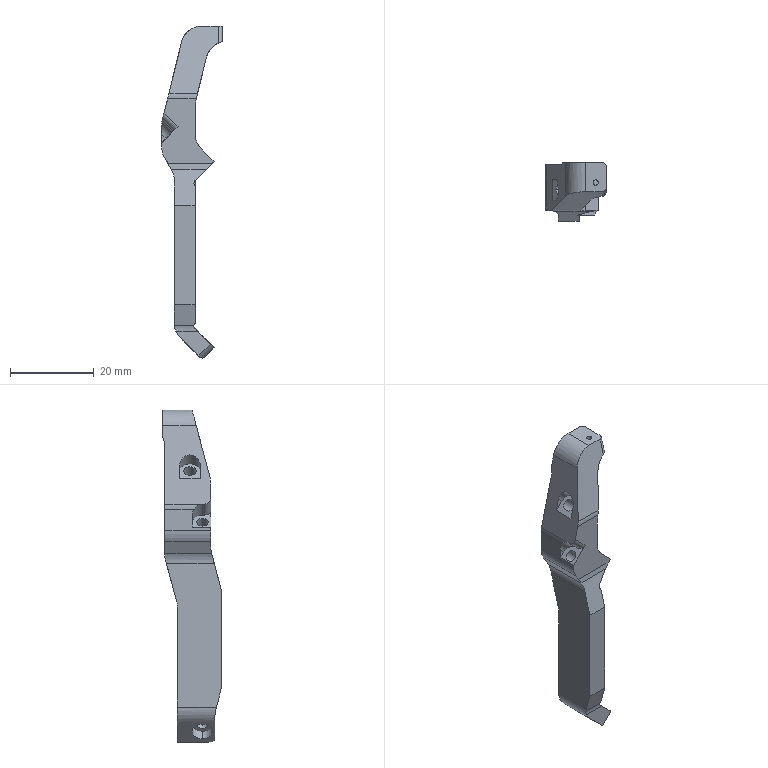NC program | NX | posted by the shop | part box 14.5 x 14 x 79.438 mm
Lines 1 to 1009 of 13169:
O001
(2026-03-11 12:15)
(DaHai UG POST QQ: 710181423)
(******************T O O L  L I S T******************)
(Tool_Num   Tool_Name          Tool_D/R    Tool_Len  )
(  T7 Drill D3.0-42-71 3.000 71.000    )
(  T8 Drill D2.7-39-67 2.700 67.000    )
(  T12 D1.3 drill 1.300 80.000    )
(  T1 D8-25-D8-60-3T-rough 8.000 60.000    )
(  T2 D6-18-D6-50-3T-rough 6.000 50.000    )
(  T4 D4-12-D4-50-3T-rough 4.000 50.000    )
(  T5 D4-12-D4-50-3T-finish 4.000 50.000    )
(  T6 Chamfer D4-90deg 4.000 50.000    )
(  T3 D6-18-D6-50-3T-finish 6.000 50.000    )
(  T9 Ball end mill R1.25-4-D4-50 2.500 4.500     )
(  T0       MILL            3.000      75.000    )
(  T11      D2-7-D2-50-3T   2.000      50.000    )
(  T13 M1.6 thread mill 1.150 50.000    )
(****************************************************)
N01
G17 G40 G80 G94
T01 M6 ( D8-25-D8-60-3T-rough )
M41
M51
G90 G54 G00 B0.0 C0.0
M40
M50
G54 G00 X50.241 Y2.792 S4500 M03
G43 H01 Z30.2 M08
Z-16.5
G01 X50.217 Y2.796 Z-16.656 F2000.
X50.192 Y2.8 Z-16.718
X50.167 Y2.804 Z-16.763
X50.143 Y2.808 Z-16.8
X50.118 Y2.812 Z-16.831
X50.093 Y2.816 Z-16.857
X50.068 Y2.819 Z-16.88
X50.044 Y2.823 Z-16.9
X50.019 Y2.827 Z-16.918
X49.994 Y2.831 Z-16.933
X49.97 Y2.835 Z-16.947
X49.945 Y2.839 Z-16.958
X49.92 Y2.843 Z-16.968
X49.896 Y2.847 Z-16.977
X49.871 Y2.85 Z-16.984
X49.846 Y2.854 Z-16.99
X49.822 Y2.858 Z-16.994
X49.797 Y2.862 Z-16.997
X49.772 Y2.866 Z-16.999
X49.747 Y2.87 Z-17.
X48.648 Y3.043
X48.523 Y3.052
G03 X47.719 Y2.326 R0.808
X47.525 Y-0.532 R21.101
X47.53 Y-1.027 R21.101
G02 X47.533 Y-2.434 R334.968
X47.499 Y-7.216 R334.968
X45.031 Y-10.745 R4.685
X41.292 Y-11.738 R8.93
X36.475 Y-11.861 R94.387
X35.02 Y-11.849 R94.387
G01 X-42.511 Y-11.85
G02 X-46.258 Y-9.609 R4.561
X-47.373 Y-5.982 R8.204
X-47.525 Y-1.714 R59.86
X-47.517 Y-0.736 R59.86
X-47.531 Y2.431 R363.519
X-47.499 Y7.213 R363.519
X-44.99 Y10.768 R4.695
X-41.419 Y11.727 R8.834
X-36.776 Y11.859 R81.431
X-35.472 Y11.849 R81.431
G01 X42.499 Y11.85
G02 X46.267 Y9.607 R4.55
X47.371 Y6.007 R8.19
X47.48 Y3.474 R29.621
X47.393 Y1.209 R29.621
G03 X47.304 Y-6.017 R363.314
G02 X44.149 Y-10.538 R5.548
X40.096 Y-11.529 R10.625
X35.197 Y-11.657 R93.798
X33.973 Y-11.649 R93.798
G01 X-41.271 Y-11.65
G02 X-46.145 Y-8.592 R5.513
X-47.182 Y-4.603 R10.225
X-47.331 Y0.65 R93.215
X-47.318 Y2.169 R93.215
X-47.331 Y3.595 R82.44
X-47.29 Y6.165 R82.44
X-44.126 Y10.549 R5.564
X-40.143 Y11.524 R10.591
X-35.291 Y11.656 R89.821
X-34.146 Y11.648 R89.821
G01 X41.26 Y11.65
G02 X46.128 Y8.629 R5.495
X47.19 Y4.395 R10.158
X47.212 Y2.636 R70.102
X47.156 Y-0.183 R70.102
X47.096 Y-5.198 R392.063
X43.437 Y-10.343 R6.159
X39.221 Y-11.32 R11.889
X34.022 Y-11.457 R98.864
X32.749 Y-11.449 R98.864
G01 X-10.796 Y-11.45
X-40.148
X-40.346 Y-11.453
G02 X-46.045 Y-7.692 R6.199
X-46.991 Y-3.519 R12.055
X-47.124 Y1.49 R94.739
X-47.117 Y2.578 R94.739
X-47.131 Y3.485 R29.603
X-47.061 Y5.526 R29.603
X-43.368 Y10.375 R6.177
X-41.602 Y10.998 R18.39
G01 X-40.654 Y11.345
X-39.718 Y11.45
X-32.765 Y11.449
X40.334 Y11.448
X40.368
G02 X46.022 Y7.745 R6.168
X46.953 Y3.298 R11.287
X46.964 Y1.098 R213.401
X46.891 Y-4.482 R213.401
X42.765 Y-10.172 R6.648
X38.337 Y-11.124 R13.258
X33.139 Y-11.254 R104.059
X32.064 Y-11.248 R104.059
G01 X-8.922 Y-11.249
G02 X-10.799 Y-11.45 R10.125
G01 X-15.974
G03 X-21.246 Y-11.245 R67.938
X-22.203 Y-11.252 R67.938
G01 X-24.798 Y-11.25
X-39.298 Y-11.249
G02 X-39.586 Y-11.255 R6.884
X-43.821 Y-9.798 R6.884
X-46.376 Y-5.505 R7.829
X-46.881 Y-0.749 R22.645
G01 Y-0.666
G02 X-46.921 Y1.965 R85.821
X-46.884 Y4.508 R85.821
X-43.109 Y10.017 R6.62
G03 X-42.521 Y10.35 R4.842
X-42.288 Y10.915 R0.8
X-42.521 Y11.48 R0.8
X-43.101 Y11.716 Z-16.96 R0.83
G01 X-43.234 Y11.705 Z-16.951
X-44.048 Y11.631 Z-16.9
X-45.501 Y11.498 F9999.
G03 X-45.983 Y11.278 R0.807
G01 X-46.461 Y10.819
X-46.932 Y10.353
G03 X-47.883 Y9.017 R6.242
G01 X-48.209 Y8.402
X-48.524 Y7.782
G03 X-49.121 Y5.797 R7.889
X-49.265 Y4.316 R10.848
G01 X-49.393 Y-0.659
G03 X-49.397 Y-1.069 R19.738
X-48.982 Y-5.096 R19.738
X-46.279 Y-10.779 R12.276
X-42.415 Y-13.222 R8.002
X-41.004 Y-13.484 R10.68
X-38.632 Y-13.653 R21.259
G01 X-19.548 Y-13.925
X-19.393 Y-13.91
X-19.242 Y-13.869
X-17.782 Y-13.29
X-16.802 Y-12.897 Z-16.966 F2000.
G03 X-16.43 Y-12.525 Z-17. R0.803
X-16.351 Y-12.179 R0.8
X-17.014 Y-11.391 R0.8
X-20.57 Y-11.067 R19.704
X-20.904 Y-11.07 R19.704
G01 X-26.448 Y-11.05
X-38.398 Y-11.049
G02 X-38.757 Y-11.057 R8.291
X-42.281 Y-10.271 R8.291
X-45.875 Y-5.928 R7.429
X-46.634 Y-1.205 R17.036
X-46.715 Y1.682 R51.49
X-46.662 Y4.017 R51.49
X-43.732 Y9.171 R7.039
G03 X-43.117 Y9.687 R4.02
X-42.984 Y10.129 R0.8
X-43.451 Y10.856 R0.8
X-43.787 Y10.926 Z-16.978 R0.84
X-44.17 Y10.834 Z-16.953 R0.84
G01 X-44.95 Y10.5 Z-16.9
X-45.749 Y10.162 F9999.
X-46.541 Y9.811
X-46.701 Y9.687
X-47.221 Y9.154
G03 X-47.635 Y8.542 R3.44
G01 X-48.315 Y7.219
X-48.518 Y6.766
X-48.69 Y6.3
X-48.807 Y5.819
X-49.071 Y4.351
G03 X-49.205 Y2.503 R12.818
X-49.19 Y1.88 R12.818
G01 X-48.945 Y-3.092
G03 X-47.902 Y-7.399 R12.181
X-46.551 Y-9.824 R16.642
X-45.251 Y-11.313 R8.364
X-43.6 Y-12.393 R7.399
X-40.567 Y-13.26 R8.637
X-37.097 Y-13.47 R42.722
G01 X-20.435 Y-13.771
X-20.278 Y-13.757
X-20.125 Y-13.715
X-18.65 Y-13.129
X-17.687 Y-12.742 Z-16.965 F2000.
G03 X-17.308 Y-12.353 Z-17. R0.802
X-17.238 Y-12.025 R0.8
X-17.901 Y-11.237 R0.8
X-21.079 Y-10.888 R14.642
G01 X-21.223 Y-10.889
G03 X-27.223 Y-10.85 R578.32
G02 X-31.319 Y-10.86 R827.506
X-38.548 Y-10.829 R827.506
X-43.845 Y-8.558 R7.442
X-46.052 Y-3.965 R9.257
X-46.486 Y1.063 R29.355
G01 Y1.16
G02 X-46.511 Y2.002 R14.097
X-46.276 Y4.569 R14.097
X-44.01 Y8.471 R7.877
G03 X-43.516 Y9.04 R3.297
X-43.453 Y9.352 R0.8
X-43.801 Y10.012 R0.8
X-44.261 Y10.15 Z-16.969 R0.832
X-44.568 Y10.092 Z-16.95 R0.832
G01 X-45.322 Y9.855 Z-16.9
X-46.624 Y9.446 F9999.
G03 X-47.1 Y9.04 R0.804
G01 X-47.637 Y7.974
X-48.158 Y6.901
G03 X-48.716 Y4.904 R8.058
X-48.85 Y3.421 R12.255
G01 X-48.895 Y1.823
X-48.922 Y0.225
G03 X-48.51 Y-3.999 R22.992
X-48.147 Y-5.645 R17.405
X-47.158 Y-8.074 R12.075
G01 X-46.86 Y-8.626
X-46.551 Y-9.171
G03 X-44.988 Y-10.946 R7.52
X-41.118 Y-12.848 R8.632
G01 X-40.483 Y-12.961
X-39.844 Y-13.046
G03 X-36.876 Y-13.274 R28.74
G01 X-20.952 Y-13.657
X-20.787 Y-13.642
X-20.628 Y-13.597
X-19.176 Y-12.999
X-18.246 Y-12.61 Z-16.963 F2000.
G03 X-17.862 Y-12.187 Z-17. R0.801
X-17.809 Y-11.9 R0.8
X-18.418 Y-11.123 R0.8
X-21.71 Y-10.703 R13.13
G01 X-21.754
G03 X-31.829 Y-10.636 R756.01
X-36.473 Y-10.65 R756.01
G02 X-37.043 Y-10.662 R13.843
X-40.048 Y-10.332 R13.843
X-45.164 Y-5.737 R7.625
X-46.162 Y-1.037 R15.078
X-46.274 Y1.27 R23.738
X-46.183 Y3.357 R23.738
X-44.311 Y7.647 R8.561
G03 X-43.693 Y8.529 R7.28
G01 X-43.503 Y9.072
X-43.003 Y9.869
X-42.338 Y10.534
X-41.576 Y11.013
G03 X-41.201 Y11.69 R0.8
X-42.001 Y12.49 R0.8
X-42.33 Y12.419 R0.8
G01 X-42.57 Y12.311
X-44.023 Y11.658 Z-16.9
X-44.475 Y11.457 F9999.
X-44.921 Y11.245
X-45.052 Y11.14
X-45.16 Y11.013
X-45.992 Y9.772
X-46.811 Y8.524
G03 X-48.645 Y3.438 R13.655
X-48.867 Y0.897 R14.666
X-48.847 Y0.127 R14.666
G01 X-48.8 Y-0.436
X-48.732 Y-0.996
X-48.521 Y-2.473
X-48.294 Y-3.948
G03 X-46.078 Y-8.865 R11.636
G01 X-45.623 Y-9.456
X-45.161 Y-10.04
G03 X-44.475 Y-10.756 R6.06
G01 X-44.279 Y-10.906
X-44.075 Y-11.046
X-43.304 Y-11.532
X-42.525 Y-12.006
G03 X-40.617 Y-12.703 R6.565
X-39.047 Y-12.893 R9.298
G01 X-21.656 Y-13.484
X-21.487 Y-13.47
X-21.323 Y-13.423
X-19.881 Y-12.827
X-18.95 Y-12.436 Z-16.964 F2000.
G03 X-18.567 Y-12.016 Z-17. R0.801
X-18.513 Y-11.726 R0.8
X-19.122 Y-10.949 R0.8
X-22.636 Y-10.502 R14.021
G01 X-22.721
G03 X-33.185 Y-10.437 R834.627
X-36.723 Y-10.444 R834.627
G02 X-36.978 Y-10.447 R10.31
X-40.78 Y-9.721 R10.31
X-45.052 Y-5.065 R8.04
X-45.991 Y-0.021 R17.013
X-46.05 Y1.214 R13.014
X-45.737 Y4.054 R13.014
X-44.184 Y7.347 R11.131
G03 X-43.836 Y8.016 R2.746
G01 X-43.821 Y8.17
G03 X-44.391 Y8.936 R0.8
X-44.618 Y8.968 Z-16.986 R0.833
X-45.143 Y8.781 Z-16.95 R0.833
G01 X-45.795 Y8.328 Z-16.9
X-46.995 Y7.492 F9999.
G03 X-47.298 Y7.089 R0.809
G01 X-47.918 Y5.199
G03 X-48.469 Y2.277 R15.69
X-48.562 Y0.585 R15.415
X-48.286 Y-2.323 R15.415
X-47.464 Y-5.527 R23.524
G01 X-47.244 Y-6.187
X-47.014 Y-6.844
G03 X-44.992 Y-9.732 R7.303
G01 X-44.373 Y-10.261
X-43.747 Y-10.783
G03 X-39.557 Y-12.716 R10.291
X-37.531 Y-12.953 R10.986
G01 X-22.433 Y-13.293
X-22.269 Y-13.278
X-22.11 Y-13.232
X-20.656 Y-12.633
X-19.727 Y-12.245 Z-16.963 F2000.
G03 X-19.343 Y-11.821 Z-17. R0.801
X-19.29 Y-11.535 R0.8
X-19.899 Y-10.758 R0.8
X-23.443 Y-10.306 R14.111
G01 X-23.502
G03 X-33.455 Y-10.237 R715.439
X-36.223 Y-10.242 R715.439
G02 X-36.452 Y-10.244 R10.898
X-40.335 Y-9.529 R10.898
X-44.782 Y-4.811 R8.21
X-45.783 Y0.904 R16.818
X-45.682 Y2.743 R16.818
X-44.246 Y6.741 R11.611
G03 X-43.814 Y8.185 R2.754
G01 X-43.69 Y8.539
G03 X-43.645 Y8.803 R0.8
X-44.267 Y9.583 R0.8
G01 X-44.439 Y9.601 Z-16.989
G03 X-44.97 Y9.411 Z-16.953 R0.839
G01 X-45.658 Y8.923 Z-16.9
X-46.834 Y8.09 F9999.
G03 X-47.152 Y7.611 R0.806
G01 X-47.845 Y4.455
G03 X-48.278 Y1.757 R30.311
X-48.324 Y0.773 R10.695
X-48.221 Y-0.709 R10.695
X-46.941 Y-6.008 R24.32
X-45.829 Y-8.213 R11.373
X-45.087 Y-9.265 R9.573
X-43.617 Y-10.582 R7.67
X-40.772 Y-11.952 R9.209
X-37.861 Y-12.516 R14.095
G01 X-37.367 Y-12.545
X-23.21 Y-13.101
X-23.038 Y-13.088
X-22.872 Y-13.041
X-21.432 Y-12.444
X-20.502 Y-12.053 Z-16.963 F2000.
G03 X-20.12 Y-11.631 Z-17. R0.801
X-20.067 Y-11.344 R0.8
X-20.675 Y-10.567 R0.8
X-24.167 Y-10.113 R13.785
X-33.012 Y-10.036 R506.58
X-35.598 Y-10.043 R506.58
G02 X-35.864 Y-10.046 R11.997
X-39.727 Y-9.407 R11.997
X-44.525 Y-4.541 R8.355
X-45.516 Y0.748 R14.609
X-45.374 Y2.779 R14.609
X-44.155 Y6.395 R14.567
G03 X-43.919 Y7.251 R1.867
G01 X-43.88 Y7.599
X-43.875 Y7.688
G03 X-44.409 Y8.443 R0.8
X-44.673 Y8.486 Z-16.983 R0.833
X-45.166 Y8.325 Z-16.95 R0.833
G01 X-45.841 Y7.904 Z-16.9
X-46.981 Y7.193 F9999.
G03 X-47.342 Y6.671 R0.804
G01 X-47.596 Y5.418
X-47.832 Y4.162
G03 X-48.011 Y1.896 R14.414
X-47.968 Y0.781 R14.414
X-47.746 Y-1.527 R34.471
X-47.06 Y-4.588 R19.689
X-45.523 Y-7.66 R11.528
X-44.15 Y-9.363 R11.997
X-42.162 Y-10.971 R13.175
X-39.214 Y-12.051 R7.207
X-34.269 Y-12.498 R54.023
G01 X-23.987 Y-12.91
X-23.814 Y-12.897
X-23.648 Y-12.85
X-22.206 Y-12.252
X-21.279 Y-11.862 Z-16.963 F2000.
G03 X-20.895 Y-11.437 Z-17. R0.801
X-20.843 Y-11.153 R0.8
X-21.452 Y-10.376 R0.8
X-24.946 Y-9.916 R13.802
X-33.892 Y-9.837 R502.098
X-35.273 Y-9.838 R502.098
G01 X-35.462 Y-9.84
G02 X-39.517 Y-9.134 R12.002
X-44.321 Y-4.153 R8.564
X-45.238 Y0.631 R12.934
X-44.957 Y3.312 R12.934
X-43.986 Y6.284 R30.242
G03 X-43.904 Y6.874 R2.161
X-43.919 Y7.126 R2.161
X-44.719 Y7.926 R0.8
G01 X-44.761 Y7.925
G03 X-45.399 Y7.555 Z-16.952 R0.838
G01 X-45.904 Y6.898 Z-16.9
X-46.881 Y5.628 F9999.
X-46.966 Y5.488
X-47.023 Y5.334
X-47.326 Y4.13
X-47.614 Y2.923
G03 X-47.829 Y0.777 R10.834
X-47.752 Y-0.506 R10.834
X-46.358 Y-5.55 R15.011
X-45.145 Y-7.714 R19.104
X-43.58 Y-9.496 R8.758
X-41.441 Y-10.894 R12.815
X-39.399 Y-11.669 R11.798
X-37.465 Y-12.079 R11.345
G01 X-36.478 Y-12.178
X-35.488 Y-12.242
X-24.788 Y-12.713
X-24.614 Y-12.7
X-24.446 Y-12.653
X-23.006 Y-12.055
X-22.08 Y-11.665 Z-16.963 F2000.
G03 X-21.696 Y-11.238 Z-17. R0.801
X-21.644 Y-10.956 R0.8
X-22.253 Y-10.179 R0.8
X-25.748 Y-9.718 R13.841
X-34.59 Y-9.635 R474.723
G01 X-34.874 Y-9.636
X-35.021
G02 X-39.167 Y-8.921 R12.371
X-44.083 Y-3.862 R8.717
X-44.947 Y0.678 R12.361
X-44.263 Y4.731 R12.361
G03 X-43.919 Y5.96 R12.763
G01 Y6.61
G03 X-44.719 Y7.41 R0.8
G01 X-44.772 Y7.408
G03 X-45.403 Y7.031 Z-16.952 R0.838
G01 X-45.904 Y6.368 Z-16.9
X-46.902 Y5.047 F9999.
X-46.97 Y4.936
X-47.023 Y4.817
X-47.234 Y4.19
X-47.431 Y3.559
G03 X-47.6 Y2.252 R5.144
X-47.59 Y1.935 R5.144
X-47.408 Y-0.377 R36.77
X-46.7 Y-3.945 R25.339
X-45.065 Y-7.29 R10.555
X-43.937 Y-8.55 R9.598
G01 X-43.273 Y-9.174
X-42.597 Y-9.788
G03 X-41.212 Y-10.655 R6.03
X-38.993 Y-11.519 R21.575
X-37.439 Y-11.799 R7.248
G01 X-33.964 Y-12.036
X-30.489 Y-12.257
X-28.039 Y-12.391
X-25.589 Y-12.516
X-25.558 Y-12.517
G03 X-25.241 Y-12.456 R0.854
G01 X-23.806 Y-11.859
X-22.88 Y-11.467 Z-16.963 F2000.
G03 X-22.497 Y-11.041 Z-17. R0.801
X-22.446 Y-10.759 R0.8
X-23.054 Y-9.982 R0.8
X-26.549 Y-9.519 R13.867
X-34.679 Y-9.427 R599.989
G01 X-34.708
G02 X-39.1 Y-8.597 R12.035
X-43.915 Y-3.395 R8.909
X-44.648 Y0.749 R12.075
X-44.181 Y4.075 R12.075
G01 X-43.919 Y5.178
Y5.978
G03 X-44.719 Y6.778 R0.8
G01 X-44.785 Y6.775
G03 X-45.408 Y6.392 Z-16.953 R0.838
G01 X-45.904 Y5.721 Z-16.9
X-46.951 Y4.304 F9999.
X-47.15 Y3.939
X-47.324 Y3.562
G03 X-47.446 Y2.888 R1.923
G01 X-47.444 Y2.798
G03 X-47.295 Y0.617 R30.389
X-46.99 Y-1.144 R17.858
G01 X-46.724 Y-2.322
X-46.444 Y-3.497
G03 X-45.451 Y-5.821 R9.419
X-44.071 Y-7.885 R17.839
X-42.648 Y-9.249 R6.985
G01 X-42.066 Y-9.666
X-41.478 Y-10.075
G03 X-38.271 Y-11.378 R9.22
X-34.335 Y-11.877 R28.239
G01 X-26.39 Y-12.319
X-26.354 Y-12.32
G03 X-26.037 Y-12.259 R0.852
G01 X-24.606 Y-11.661
X-23.681 Y-11.27 Z-16.963 F2000.
G03 X-23.298 Y-10.843 Z-17. R0.801
X-23.247 Y-10.562 R0.8
X-23.855 Y-9.785 R0.8
X-27.552 Y-9.311 R14.658
G01 X-27.597
X-34.461 Y-9.218
G02 X-39.079 Y-8.248 R11.766
X-43.837 Y-2.635 R9.102
X-44.348 Y0.816 R11.918
X-44.055 Y3.442 R11.918
G01 X-43.919 Y4.169
Y5.194
G03 X-44.714 Y5.994 R0.8
X-45.379 Y5.651 Z-16.951 R0.83
G01 X-45.904 Y5.027 Z-16.9
X-46.836 Y3.916 F9999.
G03 X-47.023 Y3.402 R0.807
G01 Y2.407
X-47.014 Y1.413
G03 X-46.701 Y-1.043 R13.805
G01 X-46.46 Y-2.148
X-46.204 Y-3.249
G03 X-44.97 Y-6.095 R10.705
X-43.151 Y-8.435 R11.967
G01 X-42.742 Y-8.843
X-42.308 Y-9.226
G03 X-41.202 Y-9.924 R5.986
X-37.466 Y-11.223 R18.266
X-35.505 Y-11.511 R16.554
X-31.541 Y-11.844 R99.631
G01 X-27.215 Y-12.116
X-27.173 Y-12.117
G03 X-26.856 Y-12.056 R0.848
G01 X-25.43 Y-11.459
X-24.505 Y-11.066 Z-16.963 F2000.
G03 X-24.123 Y-10.638 Z-17. R0.801
X-24.072 Y-10.358 R0.8
X-24.681 Y-9.582 R0.8
X-28.35 Y-9.112 R14.575
G01 X-28.382
G02 X-34.474 Y-8.997 R447.093
X-39.28 Y-7.774 R11.111
X-43.831 Y-1.369 R9.266
X-44.041 Y0.89 R12.248
X-43.919 Y2.612 R12.248
G01 Y4.187
G03 X-44.719 Y4.987 R0.8
X-45.295 Y4.742 R0.8
X-45.524 Y4.316 Z-16.969 R1.096
G01 X-45.906 Y3.28 Z-16.9
X-46.174 Y2.561 F9999.
X-46.431 Y1.84
X-46.453 Y1.653
X-46.456 Y0.659
X-46.442 Y-0.335
G03 X-45.868 Y-3.339 R11.23
X-44.741 Y-5.901 R14.4
X-42.802 Y-8.213 R9.154
X-40.369 Y-9.919 R14.822
X-37.423 Y-11.054 R9.209
G01 X-37.031 Y-11.115
X-36.638 Y-11.161
X-28.016 Y-11.919
X-27.952 Y-11.921
G03 X-27.635 Y-11.859 R0.837
G01 X-26.226 Y-11.264
X-25.304 Y-10.868 Z-16.963 F2000.
G03 X-24.922 Y-10.438 Z-17. R0.801
X-24.873 Y-10.161 R0.8
X-25.482 Y-9.384 R0.8
X-29.158 Y-8.913 R14.566
G01 X-29.183
G02 X-34.519 Y-8.766 R146.592
X-39.516 Y-7.242 R10.598
X-43.685 Y-0.115 R9.336
G03 X-43.819 Y1.01 R5.308
G01 X-43.919 Y2.613
G03 X-44.719 Y3.413 R0.8
X-45.148 Y3.288 R0.8
X-45.489 Y2.844 Z-16.964 R0.863
G01 X-45.876 Y1.898 Z-16.9
X-46.418 Y0.576 F9999.
G03 X-46.477 Y0.272 R0.81
G01 X-46.453 Y0.079
X-46.201 Y-0.935
X-45.936 Y-1.945
G03 X-44.442 Y-5.5 R17.734
X-42.635 Y-7.825 R10.796
G01 X-42.137 Y-8.311
X-41.631 Y-8.789
G03 X-38.502 Y-10.417 R7.373
X-35.982 Y-10.978 R39.162
X-33.621 Y-11.294 R27.796
G01 X-28.817 Y-11.722
X-28.752 Y-11.724
G03 X-28.435 Y-11.662 R0.836
G01 X-27.026 Y-11.066
X-26.105 Y-10.671 Z-16.963 F2000.
G03 X-25.723 Y-10.239 Z-17. R0.801
X-25.674 Y-9.964 R0.8
X-26.283 Y-9.187 R0.8
X-29.99 Y-8.712 R14.687
G01 X-30.024
G02 X-34.774 Y-8.505 R62.861
X-40.263 Y-6.254 R9.892
X-43.219 Y-1.094 R9.231
X-43.74 Y0.661 R7.435
G03 X-44.521 Y1.285 R0.8
X-45.251 Y0.812 R0.8
G01 X-45.309 Y0.615 Z-16.987
X-45.333 Y0.411 Z-16.974
X-45.455 Y-0.764 Z-16.9
X-45.589 Y-2.055 F9999.
X-45.593 Y-2.132
G03 X-45.532 Y-2.443 R0.834
G01 X-45.096 Y-3.504
X-44.644 Y-4.558
G03 X-42.824 Y-7.143 R9.259
G01 X-41.726 Y-8.229
G03 X-37.963 Y-10.361 R9.479
X-36.799 Y-10.599 R8.542
G01 X-29.643 Y-11.519
X-29.544 Y-11.525
G03 X-29.225 Y-11.46 R0.82
G01 X-27.842 Y-10.865
X-26.925 Y-10.465 Z-16.963 F2000.
G03 X-26.546 Y-10.029 Z-17. R0.801
X-26.5 Y-9.761 R0.8
X-27.108 Y-8.984 R0.8
X-30.636 Y-8.517 R14.205
G02 X-35.017 Y-8.225 R39.005
X-40.822 Y-5.203 R9.481
X-42.36 Y-2.762 R9.65
G01 X-43.031 Y-1.581
X-43.22 Y-1.092
G03 X-43.966 Y-0.58 R0.8
X-44.766 Y-1.38 R0.8
G01 X-44.759 Y-1.491
X-44.476 Y-3.059 Z-16.9
X-44.36 Y-3.715 F9999.
X-44.233 Y-4.37
X-44.148 Y-4.554
X-43.642 Y-5.365
X-43.124 Y-6.168
G03 X-41.024 Y-8.334 R9.298
X-36.558 Y-10.369 R11.136
G01 X-36.072 Y-10.455
X-30.444 Y-11.321
X-30.324 Y-11.33
G03 X-30.003 Y-11.264 R0.816
G01 X-28.639 Y-10.671
X-27.724 Y-10.266 Z-16.963 F2000.
G03 X-27.346 Y-9.829 Z-17. R0.801
X-27.301 Y-9.564 R0.8
X-27.91 Y-8.787 R0.8
X-31.166 Y-8.322 R13.784
G02 X-35.449 Y-7.882 R26.528
X-41.238 Y-4.1 R9.227
G01 X-41.522 Y-3.831
X-42.355 Y-2.768
G03 X-42.985 Y-2.461 R0.8
X-43.585 Y-2.732 R0.8
X-43.785 Y-3.277 Z-16.963 R0.842
G01 X-43.774 Y-3.411 Z-16.954
X-43.698 Y-4.272 Z-16.9
X-43.572 Y-5.682 F9999.
G03 X-43.282 Y-6.23 R0.804
X-41.468 Y-7.66 R33.626
G01 X-40.784 Y-8.129
X-40.088 Y-8.58
G03 X-37.287 Y-9.807 R12.336
X-34.979 Y-10.391 R22.488
G01 X-31.269 Y-11.118
X-31.117 Y-11.133
G03 X-30.791 Y-11.064 R0.811
G01 X-29.451 Y-10.469
X-28.543 Y-10.06 Z-16.963 F2000.
G03 X-28.168 Y-9.615 Z-17. R0.801
X-28.126 Y-9.361 R0.8
X-28.735 Y-8.584 R0.8
X-31.586 Y-8.128 R13.536
G02 X-35.826 Y-7.509 R21.14
X-39.723 Y-5.334 R9.349
X-41.244 Y-4.094 R7.756
G03 X-41.794 Y-3.875 R0.8
X-42.592 Y-4.607 R0.8
G01 Y-4.643 Z-16.998
G03 X-42.458 Y-5.149 Z-16.965 R1.02
G01 X-42.033 Y-6.084 Z-16.9
X-41.704 Y-6.807 F9999.
G03 X-41.244 Y-7.23 R0.804
G01 X-31.778 Y-10.599
G03 X-31.51 Y-10.644 R0.806
X-31.219 Y-10.59 R0.806
G01 X-30.344 Y-10.248
X-29.402 Y-9.875 Z-16.964 F2000.
G03 X-29.012 Y-9.464 Z-17. R0.801
X-28.952 Y-9.158 R0.8
X-29.56 Y-8.381 R0.8
X-32.941 Y-7.817 R20.552
G02 X-37.55 Y-6.49 R12.701
G03 X-39.424 Y-5.543 R28.873
G01 X-39.731 Y-5.328
G03 X-40.19 Y-5.184 R0.8
X-40.99 Y-5.984 R0.8
G01 X-40.967 Y-6.175
G03 X-40.718 Y-6.605 Z-16.969 R1.072
G01 X-40.036 Y-7.457 Z-16.9
X-39.18 Y-8.529 F9999.
G03 X-38.804 Y-8.79 R0.814
G01 X-32.969 Y-10.7
G03 X-32.72 Y-10.74 R0.805
X-32.376 Y-10.662 R0.805
G01 X-31.113 Y-10.061
X-30.224 Y-9.631 Z-16.962 F2000.
G03 X-29.858 Y-9.169 Z-17. R0.801
X-29.825 Y-8.943 R0.8
X-30.434 Y-8.166 R0.8
X-33.93 Y-7.455 R43.591
G02 X-36.496 Y-6.674 R13.895
X-38.106 Y-6.183 R18.834
G03 X-38.354 Y-6.144 R0.8
X-39.132 Y-6.758 R0.8
G01 X-39.152 Y-6.938 Z-16.989
G03 X-38.962 Y-7.47 Z-16.952 R0.838
G01 X-38.477 Y-8.15 Z-16.9
X-37.635 Y-9.333 F9999.
G03 X-37.179 Y-9.645 R0.807
G01 X-34.037 Y-10.437
X-33.842 Y-10.461
G03 X-33.509 Y-10.389 R0.807
G01 X-32.202 Y-9.792
X-31.303 Y-9.375 Z-16.962 F2000.
G03 X-30.931 Y-8.921 Z-17. R0.801
X-30.894 Y-8.68 R0.8
X-31.502 Y-7.903 R0.8
G01 X-36.503 Y-6.673
X-36.686 Y-6.652
G03 X-37.355 Y-6.987 R0.835
G01 X-38.421 Y-8.17 Z-16.9
G02 X-38.766 Y-8.493 R1.465 F9999.
X-39.163 Y-8.599 R0.801
X-39.607 Y-8.465 R0.801
G01 X-42.092 Y-6.808
G02 X-43.789 Y-5.167 R6.634
X-44.61 Y-3.813 R8.978
G01 X-45.046 Y-2.922
X-45.449 Y-2.017
G02 X-46.318 Y1.339 R13.863
X-46.491 Y3.607 R14.889
X-46.475 Y4.307 R14.889
G01 X-46.322 Y7.526
G02 X-44.704 Y11.866 R7.585
X-41.349 Y13.679 R5.034
G01 X-38.503 Y13.984
X-38.418 Y13.989
G02 X-37.749 Y13.629 R0.801
G01 X-37.639 Y13.462
X-36.761 Y12.132 Z-17. F2000.
X-36.621 Y11.919
X-36.474 Y11.712
G03 X-35.968 Y11.45 R0.806
X-32.271 Y11.246 R33.666
X-31.524 Y11.255 R33.666
G01 X-28.339 Y11.249
X39.36 Y11.248
G02 X39.621 Y11.253 R6.769
X44.159 Y9.507 R6.769
X46.458 Y5.037 R8.034
X46.76 Y1.16 R25.034
X46.748 Y0.403 R25.034
X46.757 Y-0.651 R66.032
X46.668 Y-4.062 R66.032
X42.265 Y-9.95 R7.03
X37.687 Y-10.917 R14.07
X31.736 Y-11.059 R124.552
X30.114 Y-11.049 R124.552
G01 X-7.769
X-7.891 Y-11.044
G03 X-8.421 Y-11.137 R1.573
G01 X-9.034 Y-11.259
G03 X-9.645 Y-11.814 R0.801
G01 X-9.786 Y-12.598 Z-16.95
X-9.913 Y-13.384 Z-16.9
X-9.95 Y-13.606 F9999.
X-9.998 Y-13.826
G02 X-10.755 Y-14.366 R0.8
G01 X-10.827 Y-14.362
X-13.138 Y-14.157
X-15.448 Y-13.934
G02 X-21.168 Y-13.011 R58.132
G01 X-28.473 Y-11.453
G02 X-36.145 Y-9.361 R70.823
G01 X-38.508 Y-8.571
G02 X-41.142 Y-7.24 R10.215
X-43.093 Y-5.708 R17.047
X-44.348 Y-4.186 R7.259
X-45.373 Y-2.252 R11.89
X-45.912 Y-0.472 R11.02
X-46.283 Y2.375 R17.161
X-46.503 Y6.846 R137.545
X-46.508 Y7.12 R7.642
X-45.91 Y10.082 R7.642
X-44.426 Y12.145 R5.985
X-43.513 Y12.907 R8.731
X-40.585 Y13.844 R5.324
G01 X-37.708 Y13.893
G02 X-36.976 Y13.462 R0.85
G01 X-36.062 Y12.157 Z-17. F2000.
X-35.863 Y11.869
X-35.651 Y11.591
G03 X-35.173 Y11.359 R0.807
X-32.108 Y11.075 R16.718
G01 X-31.913 Y11.076
X-27.389 Y11.05
X38.461 Y11.048
G02 X38.794 Y11.055 R8.121
X42.403 Y10.209 R8.121
X45.891 Y5.809 R7.362
X46.515 Y1.297 R16.636
G01 Y1.192
G02 X46.546 Y-0.6 R51.075
X46.465 Y-3.481 R51.075
X41.788 Y-9.737 R7.364
X37.083 Y-10.712 R14.828
X30.66 Y-10.861 R137.963
X28.785 Y-10.849 R137.963
G01 X-6.934 Y-10.85
G03 X-7.136 Y-10.842 R2.783
X-8.284 Y-11.09 R2.783
X-8.803 Y-11.655 R0.801
G01 X-8.833 Y-11.775
X-9.216 Y-13.321 Z-16.9
X-9.265 Y-13.519 F9999.
X-9.325 Y-13.714
G02 X-10.059 Y-14.194 R0.801
G01 X-10.076
X-11.965 Y-14.156
X-13.853 Y-14.1
G02 X-17.994 Y-13.616 R33.181
X-20.917 Y-13.027 R60.762
G01 X-33.05 Y-10.252
G02 X-37.813 Y-8.84 R39.366
G01 X-39.21 Y-8.318
G02 X-41.82 Y-6.899 R14.509
X-43.796 Y-4.979 R7.44
G01 X-44.127 Y-4.485
X-44.427 Y-3.971
X-44.78 Y-3.317
X-45.124 Y-2.657
G02 X-45.879 Y-0.652 R13.39
X-46.556 Y2.078 R37.335
X-46.754 Y4.165 R11.101
X-46.672 Y5.51 R11.101
G01 X-46.31 Y8.475
G02 X-44.485 Y11.858 R5.244
G01 X-42.938 Y13.158
G02 X-40.105 Y14.19 R4.405
X-39.494 Y14.147 R4.405
G01 X-37.551 Y13.875
G02 X-37.049 Y13.596 R0.806
G01 X-36.934 Y13.459
X-35.911 Y12.237 Z-17. F2000.
X-35.604 Y11.867
G03 X-34.532 Y11.181 R1.596
X-31.35 Y10.882 R17.065
G01 X-31.151 Y10.883
X-26.139 Y10.85
X37.636 Y10.848
G02 X38.029 Y10.856 R9.632
X41.411 Y10.243 R9.632
X45.516 Y5.752 R7.421
X46.28 Y1.082 R15.639
X46.332 Y-0.688 R30.159
X46.222 Y-3.263 R30.159
X41.479 Y-9.467 R7.611
X36.761 Y-10.489 R14.869
X30.439 Y-10.66 R117.215
X28.764 Y-10.648 R117.215
G01 X-5.72 Y-10.649
G03 X-6.12 Y-10.638 R7.493
X-7.197 Y-10.716 R7.493
G01 X-7.244 Y-10.733
G03 X-7.666 Y-11.169 R0.804
G01 X-7.876 Y-11.695
X-8.467 Y-13.174 Z-16.9
X-8.55 Y-13.381 F9999.
X-8.662 Y-13.574
G02 X-9.036 Y-13.836 R0.814
G01 X-9.39 Y-13.954
X-9.746 Y-14.062
G02 X-10.433 Y-14.141 R3.012
G01 X-10.479
X-12.148 Y-14.108
X-13.817 Y-14.059
G02 X-18.873 Y-13.397 R31.237
X-27.612 Y-11.438 R442.162
G01 X-36.36 Y-9.377
G02 X-42.707 Y-6.035 R14.189
G01 X-43.415 Y-5.347
X-44.103 Y-4.639
G02 X-45.697 Y-1.498 R7.016
X-46.267 Y1.425 R35.189
X-46.465 Y3.399 R26.834
G01 X-46.616 Y5.886
G02 X-46.632 Y6.397 R8.21
X-44.921 Y11.414 R8.21
G01 X-44.597 Y11.831
X-44.246 Y12.226
G02 X-42.816 Y13.175 R4.461
X-41.238 Y13.628 R6.436
G01 X-36.526 Y14.344
X-36.406 Y14.353
G02 X-35.622 Y13.709 R0.8
G01 X-35.566 Y13.431
X-35.256 Y11.868 Z-17. F2000.
G03 X-34.734 Y11.24 R0.803
X-32.195 Y10.762 R8.031
X-26.496 Y10.64 R133.266
X-24.914 Y10.65 R133.266
G01 X36.836 Y10.648
G02 X37.281 Y10.657 R11.541
X40.516 Y10.194 R11.541
X45.222 Y5.485 R7.583
X46.05 Y0.827 R15.541
X46.11 Y-0.683 R19.041
X45.928 Y-3.312 R19.041
X41.071 Y-9.25 R7.838
X36.153 Y-10.292 R15.597
X29.778 Y-10.459 R121.814
X28.156 Y-10.448 R121.814
G01 X-4.795 Y-10.449
G03 X-5.325 Y-10.435 R10.432
X-6.858 Y-10.548 R10.432
G02 X-7.732 Y-10.903 R5.753
G03 X-8.249 Y-11.461 R0.801
G01 X-8.305 Y-11.676
X-8.701 Y-13.219 Z-16.9
G02 X-8.855 Y-13.646 R1.322 F9999.
X-9.524 Y-14.007 R0.801
G01 X-11.681 Y-14.009
X-13.837 Y-13.995
G02 X-17.948 Y-13.583 R29.105
X-22.825 Y-12.619 R106.073
G01 X-32.059 Y-10.563
G02 X-37.772 Y-8.867 R43.053
G01 X-38.469 Y-8.606
X-39.163 Y-8.336
G02 X-42.097 Y-6.544 R11.662
G01 X-42.63 Y-6.098
X-43.157 Y-5.644
G02 X-45.16 Y-2.727 R8.157
X-46.039 Y0.099 R13.483
X-46.415 Y2.98 R35.137
X-46.476 Y4.58 R21.21
X-46.387 Y6.513 R21.21
G01 X-46.205 Y8.498
G02 X-43.962 Y12.531 R5.781
X-42.503 Y13.376 R7.409
X-39.713 Y14.032 R7.729
G01 X-36.103 Y14.192
X-36.067 Y14.193
G02 X-35.29 Y13.583 R0.8
G01 X-35.244 Y13.395
X-34.866 Y11.847 Z-17. F2000.
G03 X-34.716 Y11.411 R1.353
X-34.311 Y11.088 R0.808
X-31.786 Y10.584 R7.868
X-26.199 Y10.442 R109.988